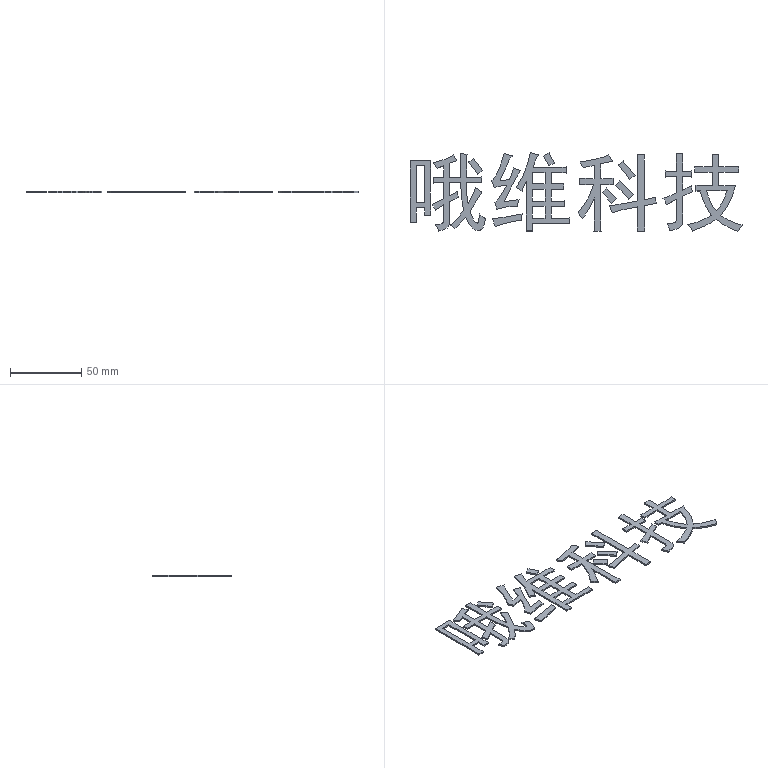Part | STEP file | COMPANY_A 01001 | 14 solids | 259 faces | box 232.982 x 55.205 x 1 mm | volume 4335 mm3 | spline 139 | plane 120